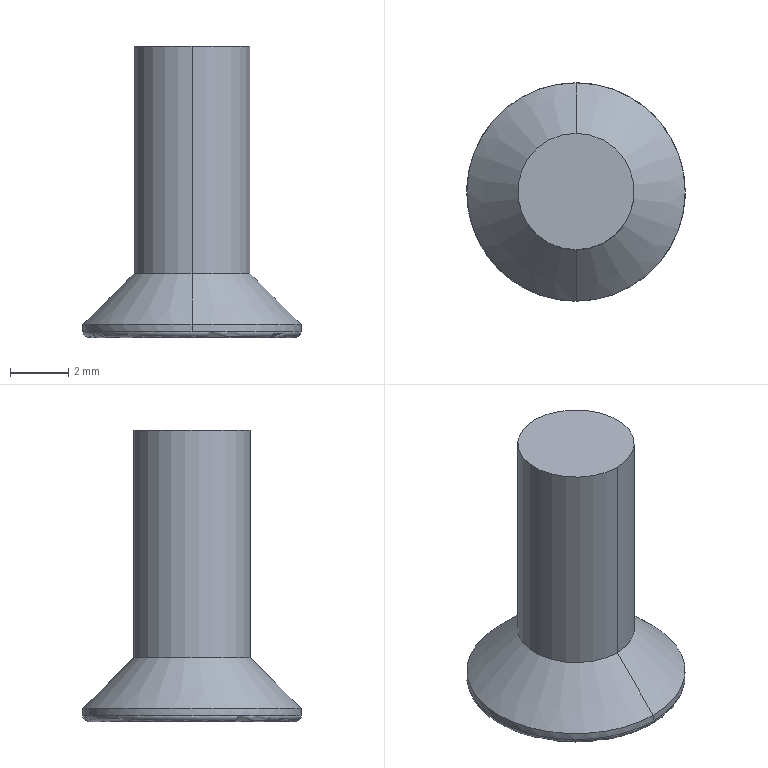Part | STEP file | ASND-0110-0162156729 | 1 solid | 23 faces | box 7.5 x 7.5 x 10 mm | volume 160.064 mm3 | plane 15 | cylinder 4 | cone 2 | torus 2 | commonest cylinder face diameters 4 x2 7.5 x2